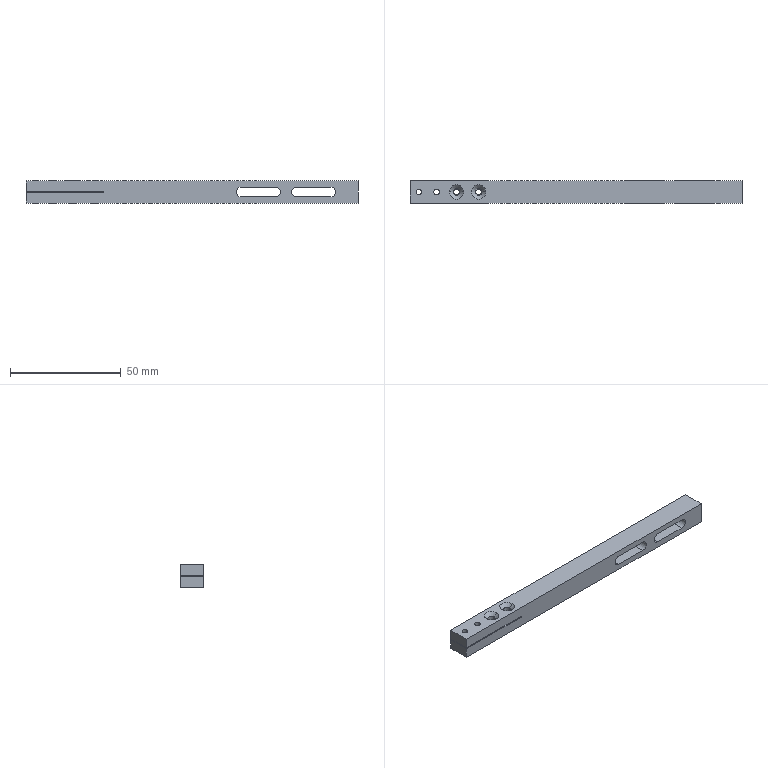Part | NX | features BREP 1 | 1 solid | 38 faces | box 150 x 10 x 10 mm | volume 12850 mm3 | cylinder 20 | plane 14 | cone 4 | commonest cylinder face diameters 2.5 x12 3.4 x4 4.5 x4
STEP:
#1=CARTESIAN_POINT('',(-64.25,0.,0.25));
#2=VERTEX_POINT('',#1);
#3=CARTESIAN_POINT('',(-61.75,0.,0.25));
#4=VERTEX_POINT('',#3);
#5=CARTESIAN_POINT('',(-63.,0.,0.25));
#6=DIRECTION('',(0.,0.,1.));
#7=DIRECTION('',(1.,0.,0.));
#8=AXIS2_PLACEMENT_3D('',#5,#6,#7);
#9=CIRCLE('',#8,1.25);
#10=EDGE_CURVE('',#2,#4,#9,.T.);
#11=ORIENTED_EDGE('',*,*,#10,.F.);
#12=CARTESIAN_POINT('',(-64.25,0.,5.));
#13=VERTEX_POINT('',#12);
#14=CARTESIAN_POINT('',(-64.25,0.,5.));
#15=DIRECTION('',(0.,0.,1.));
#16=VECTOR('',#15,1000.);
#17=LINE('',#14,#16);
#18=EDGE_CURVE('',#2,#13,#17,.T.);
#19=ORIENTED_EDGE('',*,*,#18,.T.);
#20=CARTESIAN_POINT('',(-61.75,0.,5.));
#21=VERTEX_POINT('',#20);
#22=CARTESIAN_POINT('',(-63.,0.,5.));
#23=DIRECTION('',(0.,0.,1.));
#24=DIRECTION('',(1.,0.,0.));
#25=AXIS2_PLACEMENT_3D('',#22,#23,#24);
#26=CIRCLE('',#25,1.25);
#27=EDGE_CURVE('',#13,#21,#26,.T.);
#28=ORIENTED_EDGE('',*,*,#27,.T.);
#29=CARTESIAN_POINT('',(-61.75,0.,5.));
#30=DIRECTION('',(0.,0.,1.));
#31=VECTOR('',#30,1000.);
#32=LINE('',#29,#31);
#33=EDGE_CURVE('',#4,#21,#32,.T.);
#34=ORIENTED_EDGE('',*,*,#33,.F.);
#35=EDGE_LOOP('',(#11,#19,#28,#34));
#36=FACE_BOUND('',#35,.T.);
#37=CARTESIAN_POINT('',(-63.,0.,5.));
#38=DIRECTION('',(0.,0.,1.));
#39=DIRECTION('',(-1.,0.,0.));
#40=AXIS2_PLACEMENT_3D('',#37,#38,#39);
#41=CYLINDRICAL_SURFACE('',#40,1.25);
#42=ADVANCED_FACE('',(#36),#41,.F.);
#43=CARTESIAN_POINT('',(-64.25,0.,-5.));
#44=VERTEX_POINT('',#43);
#45=CARTESIAN_POINT('',(-61.75,0.,-5.));
#46=VERTEX_POINT('',#45);
#47=CARTESIAN_POINT('',(-63.,0.,-5.));
#48=DIRECTION('',(0.,0.,1.));
#49=DIRECTION('',(1.,0.,0.));
#50=AXIS2_PLACEMENT_3D('',#47,#48,#49);
#51=CIRCLE('',#50,1.25);
#52=EDGE_CURVE('',#44,#46,#51,.T.);
#53=ORIENTED_EDGE('',*,*,#52,.F.);
#54=CARTESIAN_POINT('',(-64.25,0.,-0.25));
#55=VERTEX_POINT('',#54);
#56=CARTESIAN_POINT('',(-64.25,0.,5.));
#57=DIRECTION('',(0.,0.,1.));
#58=VECTOR('',#57,1000.);
#59=LINE('',#56,#58);
#60=EDGE_CURVE('',#44,#55,#59,.T.);
#61=ORIENTED_EDGE('',*,*,#60,.T.);
#62=CARTESIAN_POINT('',(-61.75,0.,-0.25));
#63=VERTEX_POINT('',#62);
#64=CARTESIAN_POINT('',(-63.,0.,-0.25));
#65=DIRECTION('',(0.,0.,-1.));
#66=DIRECTION('',(-1.,0.,0.));
#67=AXIS2_PLACEMENT_3D('',#64,#65,#66);
#68=CIRCLE('',#67,1.25);
#69=EDGE_CURVE('',#63,#55,#68,.T.);
#70=ORIENTED_EDGE('',*,*,#69,.F.);
#71=CARTESIAN_POINT('',(-61.75,0.,5.));
#72=DIRECTION('',(0.,0.,1.));
#73=VECTOR('',#72,1000.);
#74=LINE('',#71,#73);
#75=EDGE_CURVE('',#46,#63,#74,.T.);
#76=ORIENTED_EDGE('',*,*,#75,.F.);
#77=EDGE_LOOP('',(#53,#61,#70,#76));
#78=FACE_BOUND('',#77,.T.);
#79=CARTESIAN_POINT('',(-63.,0.,5.));
#80=DIRECTION('',(0.,0.,1.));
#81=DIRECTION('',(-1.,0.,0.));
#82=AXIS2_PLACEMENT_3D('',#79,#80,#81);
#83=CYLINDRICAL_SURFACE('',#82,1.25);
#84=ADVANCED_FACE('',(#78),#83,.F.);
#85=CARTESIAN_POINT('',(-72.25,0.,0.25));
#86=VERTEX_POINT('',#85);
#87=CARTESIAN_POINT('',(-69.75,0.,0.25));
#88=VERTEX_POINT('',#87);
#89=CARTESIAN_POINT('',(-71.,0.,0.25));
#90=DIRECTION('',(0.,0.,1.));
#91=DIRECTION('',(1.,0.,0.));
#92=AXIS2_PLACEMENT_3D('',#89,#90,#91);
#93=CIRCLE('',#92,1.25);
#94=EDGE_CURVE('',#86,#88,#93,.T.);
#95=ORIENTED_EDGE('',*,*,#94,.F.);
#96=CARTESIAN_POINT('',(-72.25,0.,5.));
#97=VERTEX_POINT('',#96);
#98=CARTESIAN_POINT('',(-72.25,0.,5.));
#99=DIRECTION('',(0.,0.,1.));
#100=VECTOR('',#99,1000.);
#101=LINE('',#98,#100);
#102=EDGE_CURVE('',#86,#97,#101,.T.);
#103=ORIENTED_EDGE('',*,*,#102,.T.);
#104=CARTESIAN_POINT('',(-69.75,0.,5.));
#105=VERTEX_POINT('',#104);
#106=CARTESIAN_POINT('',(-71.,0.,5.));
#107=DIRECTION('',(0.,0.,1.));
#108=DIRECTION('',(1.,0.,0.));
#109=AXIS2_PLACEMENT_3D('',#106,#107,#108);
#110=CIRCLE('',#109,1.25);
#111=EDGE_CURVE('',#97,#105,#110,.T.);
#112=ORIENTED_EDGE('',*,*,#111,.T.);
#113=CARTESIAN_POINT('',(-69.75,0.,5.));
#114=DIRECTION('',(0.,0.,1.));
#115=VECTOR('',#114,1000.);
#116=LINE('',#113,#115);
#117=EDGE_CURVE('',#88,#105,#116,.T.);
#118=ORIENTED_EDGE('',*,*,#117,.F.);
#119=EDGE_LOOP('',(#95,#103,#112,#118));
#120=FACE_BOUND('',#119,.T.);
#121=CARTESIAN_POINT('',(-71.,0.,5.));
#122=DIRECTION('',(0.,0.,1.));
#123=DIRECTION('',(-1.,0.,0.));
#124=AXIS2_PLACEMENT_3D('',#121,#122,#123);
#125=CYLINDRICAL_SURFACE('',#124,1.25);
#126=ADVANCED_FACE('',(#120),#125,.F.);
#127=CARTESIAN_POINT('',(-72.25,0.,-5.));
#128=VERTEX_POINT('',#127);
#129=CARTESIAN_POINT('',(-69.75,0.,-5.));
#130=VERTEX_POINT('',#129);
#131=CARTESIAN_POINT('',(-71.,0.,-5.));
#132=DIRECTION('',(0.,0.,1.));
#133=DIRECTION('',(1.,0.,0.));
#134=AXIS2_PLACEMENT_3D('',#131,#132,#133);
#135=CIRCLE('',#134,1.25);
#136=EDGE_CURVE('',#128,#130,#135,.T.);
#137=ORIENTED_EDGE('',*,*,#136,.F.);
#138=CARTESIAN_POINT('',(-72.25,0.,-0.25));
#139=VERTEX_POINT('',#138);
#140=CARTESIAN_POINT('',(-72.25,0.,5.));
#141=DIRECTION('',(0.,0.,1.));
#142=VECTOR('',#141,1000.);
#143=LINE('',#140,#142);
#144=EDGE_CURVE('',#128,#139,#143,.T.);
#145=ORIENTED_EDGE('',*,*,#144,.T.);
#146=CARTESIAN_POINT('',(-69.75,0.,-0.25));
#147=VERTEX_POINT('',#146);
#148=CARTESIAN_POINT('',(-71.,0.,-0.25));
#149=DIRECTION('',(0.,0.,-1.));
#150=DIRECTION('',(-1.,0.,0.));
#151=AXIS2_PLACEMENT_3D('',#148,#149,#150);
#152=CIRCLE('',#151,1.25);
#153=EDGE_CURVE('',#147,#139,#152,.T.);
#154=ORIENTED_EDGE('',*,*,#153,.F.);
#155=CARTESIAN_POINT('',(-69.75,0.,5.));
#156=DIRECTION('',(0.,0.,1.));
#157=VECTOR('',#156,1000.);
#158=LINE('',#155,#157);
#159=EDGE_CURVE('',#130,#147,#158,.T.);
#160=ORIENTED_EDGE('',*,*,#159,.F.);
#161=EDGE_LOOP('',(#137,#145,#154,#160));
#162=FACE_BOUND('',#161,.T.);
#163=CARTESIAN_POINT('',(-71.,0.,5.));
#164=DIRECTION('',(0.,0.,1.));
#165=DIRECTION('',(-1.,0.,0.));
#166=AXIS2_PLACEMENT_3D('',#163,#164,#165);
#167=CYLINDRICAL_SURFACE('',#166,1.25);
#168=ADVANCED_FACE('',(#162),#167,.F.);
#169=CARTESIAN_POINT('',(-55.25,0.,-5.));
#170=VERTEX_POINT('',#169);
#171=CARTESIAN_POINT('',(-52.75,0.,-5.));
#172=VERTEX_POINT('',#171);
#173=CARTESIAN_POINT('',(-54.,0.,-5.));
#174=DIRECTION('',(0.,0.,1.));
#175=DIRECTION('',(1.,0.,0.));
#176=AXIS2_PLACEMENT_3D('',#173,#174,#175);
#177=CIRCLE('',#176,1.25);
#178=EDGE_CURVE('',#170,#172,#177,.T.);
#179=ORIENTED_EDGE('',*,*,#178,.F.);
#180=CARTESIAN_POINT('',(-55.25,0.,-0.25));
#181=VERTEX_POINT('',#180);
#182=CARTESIAN_POINT('',(-55.25,0.,5.));
#183=DIRECTION('',(0.,0.,1.));
#184=VECTOR('',#183,1000.);
#185=LINE('',#182,#184);
#186=EDGE_CURVE('',#170,#181,#185,.T.);
#187=ORIENTED_EDGE('',*,*,#186,.T.);
#188=CARTESIAN_POINT('',(-52.75,0.,-0.25));
#189=VERTEX_POINT('',#188);
#190=CARTESIAN_POINT('',(-54.,0.,-0.25));
#191=DIRECTION('',(0.,0.,-1.));
#192=DIRECTION('',(-1.,0.,0.));
#193=AXIS2_PLACEMENT_3D('',#190,#191,#192);
#194=CIRCLE('',#193,1.25);
#195=EDGE_CURVE('',#189,#181,#194,.T.);
#196=ORIENTED_EDGE('',*,*,#195,.F.);
#197=CARTESIAN_POINT('',(-52.75,0.,5.));
#198=DIRECTION('',(0.,0.,1.));
#199=VECTOR('',#198,1000.);
#200=LINE('',#197,#199);
#201=EDGE_CURVE('',#172,#189,#200,.T.);
#202=ORIENTED_EDGE('',*,*,#201,.F.);
#203=EDGE_LOOP('',(#179,#187,#196,#202));
#204=FACE_BOUND('',#203,.T.);
#205=CARTESIAN_POINT('',(-54.,0.,5.));
#206=DIRECTION('',(0.,0.,1.));
#207=DIRECTION('',(-1.,0.,0.));
#208=AXIS2_PLACEMENT_3D('',#205,#206,#207);
#209=CYLINDRICAL_SURFACE('',#208,1.25);
#210=ADVANCED_FACE('',(#204),#209,.F.);
#211=CARTESIAN_POINT('',(-45.25,0.,-5.));
#212=VERTEX_POINT('',#211);
#213=CARTESIAN_POINT('',(-42.75,0.,-5.));
#214=VERTEX_POINT('',#213);
#215=CARTESIAN_POINT('',(-44.,0.,-5.));
#216=DIRECTION('',(0.,0.,1.));
#217=DIRECTION('',(1.,0.,0.));
#218=AXIS2_PLACEMENT_3D('',#215,#216,#217);
#219=CIRCLE('',#218,1.25);
#220=EDGE_CURVE('',#212,#214,#219,.T.);
#221=ORIENTED_EDGE('',*,*,#220,.F.);
#222=CARTESIAN_POINT('',(-45.25,0.,-0.25));
#223=VERTEX_POINT('',#222);
#224=CARTESIAN_POINT('',(-45.25,0.,5.));
#225=DIRECTION('',(0.,0.,1.));
#226=VECTOR('',#225,1000.);
#227=LINE('',#224,#226);
#228=EDGE_CURVE('',#212,#223,#227,.T.);
#229=ORIENTED_EDGE('',*,*,#228,.T.);
#230=CARTESIAN_POINT('',(-42.75,0.,-0.25));
#231=VERTEX_POINT('',#230);
#232=CARTESIAN_POINT('',(-44.,0.,-0.25));
#233=DIRECTION('',(0.,0.,-1.));
#234=DIRECTION('',(-1.,0.,0.));
#235=AXIS2_PLACEMENT_3D('',#232,#233,#234);
#236=CIRCLE('',#235,1.25);
#237=EDGE_CURVE('',#231,#223,#236,.T.);
#238=ORIENTED_EDGE('',*,*,#237,.F.);
#239=CARTESIAN_POINT('',(-42.75,0.,5.));
#240=DIRECTION('',(0.,0.,1.));
#241=VECTOR('',#240,1000.);
#242=LINE('',#239,#241);
#243=EDGE_CURVE('',#214,#231,#242,.T.);
#244=ORIENTED_EDGE('',*,*,#243,.F.);
#245=EDGE_LOOP('',(#221,#229,#238,#244));
#246=FACE_BOUND('',#245,.T.);
#247=CARTESIAN_POINT('',(-44.,0.,5.));
#248=DIRECTION('',(0.,0.,1.));
#249=DIRECTION('',(-1.,0.,0.));
#250=AXIS2_PLACEMENT_3D('',#247,#248,#249);
#251=CYLINDRICAL_SURFACE('',#250,1.25);
#252=ADVANCED_FACE('',(#246),#251,.F.);
#253=CARTESIAN_POINT('',(-55.7,0.,3.4));
#254=VERTEX_POINT('',#253);
#255=CARTESIAN_POINT('',(-52.3,0.,3.4));
#256=VERTEX_POINT('',#255);
#257=CARTESIAN_POINT('',(-54.,0.,3.4));
#258=DIRECTION('',(0.,0.,1.));
#259=DIRECTION('',(1.,0.,0.));
#260=AXIS2_PLACEMENT_3D('',#257,#258,#259);
#261=CIRCLE('',#260,1.7);
#262=EDGE_CURVE('',#254,#256,#261,.T.);
#263=ORIENTED_EDGE('',*,*,#262,.F.);
#264=CARTESIAN_POINT('',(-57.3,0.,5.));
#265=VERTEX_POINT('',#264);
#266=CARTESIAN_POINT('',(-57.3,0.,5.));
#267=DIRECTION('',(-0.7071,0.,0.7071));
#268=VECTOR('',#267,1000.);
#269=LINE('',#266,#268);
#270=EDGE_CURVE('',#254,#265,#269,.T.);
#271=ORIENTED_EDGE('',*,*,#270,.T.);
#272=CARTESIAN_POINT('',(-50.7,0.,5.));
#273=VERTEX_POINT('',#272);
#274=CARTESIAN_POINT('',(-54.,0.,5.));
#275=DIRECTION('',(0.,0.,1.));
#276=DIRECTION('',(1.,0.,0.));
#277=AXIS2_PLACEMENT_3D('',#274,#275,#276);
#278=CIRCLE('',#277,3.3);
#279=EDGE_CURVE('',#265,#273,#278,.T.);
#280=ORIENTED_EDGE('',*,*,#279,.T.);
#281=CARTESIAN_POINT('',(-50.7,0.,5.));
#282=DIRECTION('',(0.7071,0.,0.7071));
#283=VECTOR('',#282,1000.);
#284=LINE('',#281,#283);
#285=EDGE_CURVE('',#256,#273,#284,.T.);
#286=ORIENTED_EDGE('',*,*,#285,.F.);
#287=EDGE_LOOP('',(#263,#271,#280,#286));
#288=FACE_BOUND('',#287,.T.);
#289=CARTESIAN_POINT('',(-54.,0.,5.));
#290=DIRECTION('',(0.,0.,1.));
#291=DIRECTION('',(-1.,0.,0.));
#292=AXIS2_PLACEMENT_3D('',#289,#290,#291);
#293=CONICAL_SURFACE('',#292,3.3,0.7854);
#294=ADVANCED_FACE('',(#288),#293,.F.);
#295=CARTESIAN_POINT('',(-55.7,0.,0.25));
#296=VERTEX_POINT('',#295);
#297=CARTESIAN_POINT('',(-52.3,0.,0.25));
#298=VERTEX_POINT('',#297);
#299=CARTESIAN_POINT('',(-54.,0.,0.25));
#300=DIRECTION('',(0.,0.,1.));
#301=DIRECTION('',(1.,0.,0.));
#302=AXIS2_PLACEMENT_3D('',#299,#300,#301);
#303=CIRCLE('',#302,1.7);
#304=EDGE_CURVE('',#296,#298,#303,.T.);
#305=ORIENTED_EDGE('',*,*,#304,.F.);
#306=CARTESIAN_POINT('',(-55.7,0.,5.));
#307=DIRECTION('',(0.,0.,1.));
#308=VECTOR('',#307,1000.);
#309=LINE('',#306,#308);
#310=EDGE_CURVE('',#296,#254,#309,.T.);
#311=ORIENTED_EDGE('',*,*,#310,.T.);
#312=ORIENTED_EDGE('',*,*,#262,.T.);
#313=CARTESIAN_POINT('',(-52.3,0.,5.));
#314=DIRECTION('',(0.,0.,1.));
#315=VECTOR('',#314,1000.);
#316=LINE('',#313,#315);
#317=EDGE_CURVE('',#298,#256,#316,.T.);
#318=ORIENTED_EDGE('',*,*,#317,.F.);
#319=EDGE_LOOP('',(#305,#311,#312,#318));
#320=FACE_BOUND('',#319,.T.);
#321=CARTESIAN_POINT('',(-54.,0.,5.));
#322=DIRECTION('',(0.,0.,1.));
#323=DIRECTION('',(-1.,0.,0.));
#324=AXIS2_PLACEMENT_3D('',#321,#322,#323);
#325=CYLINDRICAL_SURFACE('',#324,1.7);
#326=ADVANCED_FACE('',(#320),#325,.F.);
#327=CARTESIAN_POINT('',(-45.7,0.,3.4));
#328=VERTEX_POINT('',#327);
#329=CARTESIAN_POINT('',(-42.3,0.,3.4));
#330=VERTEX_POINT('',#329);
#331=CARTESIAN_POINT('',(-44.,0.,3.4));
#332=DIRECTION('',(0.,0.,1.));
#333=DIRECTION('',(1.,0.,0.));
#334=AXIS2_PLACEMENT_3D('',#331,#332,#333);
#335=CIRCLE('',#334,1.7);
#336=EDGE_CURVE('',#328,#330,#335,.T.);
#337=ORIENTED_EDGE('',*,*,#336,.F.);
#338=CARTESIAN_POINT('',(-47.3,0.,5.));
#339=VERTEX_POINT('',#338);
#340=CARTESIAN_POINT('',(-47.3,0.,5.));
#341=DIRECTION('',(-0.7071,0.,0.7071));
#342=VECTOR('',#341,1000.);
#343=LINE('',#340,#342);
#344=EDGE_CURVE('',#328,#339,#343,.T.);
#345=ORIENTED_EDGE('',*,*,#344,.T.);
#346=CARTESIAN_POINT('',(-40.7,0.,5.));
#347=VERTEX_POINT('',#346);
#348=CARTESIAN_POINT('',(-44.,0.,5.));
#349=DIRECTION('',(0.,0.,1.));
#350=DIRECTION('',(1.,0.,0.));
#351=AXIS2_PLACEMENT_3D('',#348,#349,#350);
#352=CIRCLE('',#351,3.3);
#353=EDGE_CURVE('',#339,#347,#352,.T.);
#354=ORIENTED_EDGE('',*,*,#353,.T.);
#355=CARTESIAN_POINT('',(-40.7,0.,5.));
#356=DIRECTION('',(0.7071,0.,0.7071));
#357=VECTOR('',#356,1000.);
#358=LINE('',#355,#357);
#359=EDGE_CURVE('',#330,#347,#358,.T.);
#360=ORIENTED_EDGE('',*,*,#359,.F.);
#361=EDGE_LOOP('',(#337,#345,#354,#360));
#362=FACE_BOUND('',#361,.T.);
#363=CARTESIAN_POINT('',(-44.,0.,5.));
#364=DIRECTION('',(0.,0.,1.));
#365=DIRECTION('',(-1.,0.,0.));
#366=AXIS2_PLACEMENT_3D('',#363,#364,#365);
#367=CONICAL_SURFACE('',#366,3.3,0.7854);
#368=ADVANCED_FACE('',(#362),#367,.F.);
#369=CARTESIAN_POINT('',(-45.7,0.,0.25));
#370=VERTEX_POINT('',#369);
#371=CARTESIAN_POINT('',(-42.3,0.,0.25));
#372=VERTEX_POINT('',#371);
#373=CARTESIAN_POINT('',(-44.,0.,0.25));
#374=DIRECTION('',(0.,0.,1.));
#375=DIRECTION('',(1.,0.,0.));
#376=AXIS2_PLACEMENT_3D('',#373,#374,#375);
#377=CIRCLE('',#376,1.7);
#378=EDGE_CURVE('',#370,#372,#377,.T.);
#379=ORIENTED_EDGE('',*,*,#378,.F.);
#380=CARTESIAN_POINT('',(-45.7,0.,5.));
#381=DIRECTION('',(0.,0.,1.));
#382=VECTOR('',#381,1000.);
#383=LINE('',#380,#382);
#384=EDGE_CURVE('',#370,#328,#383,.T.);
#385=ORIENTED_EDGE('',*,*,#384,.T.);
#386=ORIENTED_EDGE('',*,*,#336,.T.);
#387=CARTESIAN_POINT('',(-42.3,0.,5.));
#388=DIRECTION('',(0.,0.,1.));
#389=VECTOR('',#388,1000.);
#390=LINE('',#387,#389);
#391=EDGE_CURVE('',#372,#330,#390,.T.);
#392=ORIENTED_EDGE('',*,*,#391,.F.);
#393=EDGE_LOOP('',(#379,#385,#386,#392));
#394=FACE_BOUND('',#393,.T.);
#395=CARTESIAN_POINT('',(-44.,0.,5.));
#396=DIRECTION('',(0.,0.,1.));
#397=DIRECTION('',(-1.,0.,0.));
#398=AXIS2_PLACEMENT_3D('',#395,#396,#397);
#399=CYLINDRICAL_SURFACE('',#398,1.7);
#400=ADVANCED_FACE('',(#394),#399,.F.);
#401=CARTESIAN_POINT('',(47.25,5.,2.25));
#402=VERTEX_POINT('',#401);
#403=CARTESIAN_POINT('',(62.75,5.,2.25));
#404=VERTEX_POINT('',#403);
#405=CARTESIAN_POINT('',(47.25,5.,2.25));
#406=DIRECTION('',(1.,0.,0.));
#407=VECTOR('',#406,1000.);
#408=LINE('',#405,#407);
#409=EDGE_CURVE('',#402,#404,#408,.T.);
#410=ORIENTED_EDGE('',*,*,#409,.F.);
#411=CARTESIAN_POINT('',(47.25,5.,-2.25));
#412=VERTEX_POINT('',#411);
#413=CARTESIAN_POINT('',(47.25,5.,0.));
#414=DIRECTION('',(0.,1.,0.));
#415=DIRECTION('',(0.,0.,1.));
#416=AXIS2_PLACEMENT_3D('',#413,#414,#415);
#417=CIRCLE('',#416,2.25);
#418=EDGE_CURVE('',#412,#402,#417,.T.);
#419=ORIENTED_EDGE('',*,*,#418,.F.);
#420=CARTESIAN_POINT('',(62.75,5.,-2.25));
#421=VERTEX_POINT('',#420);
#422=CARTESIAN_POINT('',(47.25,5.,-2.25));
#423=DIRECTION('',(1.,0.,0.));
#424=VECTOR('',#423,1000.);
#425=LINE('',#422,#424);
#426=EDGE_CURVE('',#412,#421,#425,.T.);
#427=ORIENTED_EDGE('',*,*,#426,.T.);
#428=CARTESIAN_POINT('',(62.75,5.,0.));
#429=DIRECTION('',(0.,1.,0.));
#430=DIRECTION('',(0.,0.,1.));
#431=AXIS2_PLACEMENT_3D('',#428,#429,#430);
#432=CIRCLE('',#431,2.25);
#433=EDGE_CURVE('',#404,#421,#432,.T.);
#434=ORIENTED_EDGE('',*,*,#433,.F.);
#435=EDGE_LOOP('',(#410,#419,#427,#434));
#436=FACE_BOUND('',#435,.T.);
#437=CARTESIAN_POINT('',(-75.,5.,-0.25));
#438=VERTEX_POINT('',#437);
#439=CARTESIAN_POINT('',(-75.,5.,-5.));
#440=VERTEX_POINT('',#439);
#441=CARTESIAN_POINT('',(-75.,5.,5.));
#442=DIRECTION('',(0.,0.,-1.));
#443=VECTOR('',#442,1000.);
#444=LINE('',#441,#443);
#445=EDGE_CURVE('',#438,#440,#444,.T.);
#446=ORIENTED_EDGE('',*,*,#445,.F.);
#447=CARTESIAN_POINT('',(-40.,5.,-0.25));
#448=VERTEX_POINT('',#447);
#449=CARTESIAN_POINT('',(-75.,5.,-0.25));
#450=DIRECTION('',(1.,0.,0.));
#451=VECTOR('',#450,1000.);
#452=LINE('',#449,#451);
#453=EDGE_CURVE('',#438,#448,#452,.T.);
#454=ORIENTED_EDGE('',*,*,#453,.T.);
#455=CARTESIAN_POINT('',(-40.,5.,0.25));
#456=VERTEX_POINT('',#455);
#457=CARTESIAN_POINT('',(-40.,5.,5.));
#458=DIRECTION('',(0.,0.,1.));
#459=VECTOR('',#458,1000.);
#460=LINE('',#457,#459);
#461=EDGE_CURVE('',#448,#456,#460,.T.);
#462=ORIENTED_EDGE('',*,*,#461,.T.);
#463=CARTESIAN_POINT('',(-75.,5.,0.25));
#464=VERTEX_POINT('',#463);
#465=CARTESIAN_POINT('',(-75.,5.,0.25));
#466=DIRECTION('',(-1.,0.,0.));
#467=VECTOR('',#466,1000.);
#468=LINE('',#465,#467);
#469=EDGE_CURVE('',#456,#464,#468,.T.);
#470=ORIENTED_EDGE('',*,*,#469,.T.);
#471=CARTESIAN_POINT('',(-75.,5.,5.));
#472=VERTEX_POINT('',#471);
#473=CARTESIAN_POINT('',(-75.,5.,5.));
#474=DIRECTION('',(0.,0.,-1.));
#475=VECTOR('',#474,1000.);
#476=LINE('',#473,#475);
#477=EDGE_CURVE('',#472,#464,#476,.T.);
#478=ORIENTED_EDGE('',*,*,#477,.F.);
#479=CARTESIAN_POINT('',(75.,5.,5.));
#480=VERTEX_POINT('',#479);
#481=CARTESIAN_POINT('',(-75.,5.,5.));
#482=DIRECTION('',(-1.,0.,0.));
#483=VECTOR('',#482,1000.);
#484=LINE('',#481,#483);
#485=EDGE_CURVE('',#480,#472,#484,.T.);
#486=ORIENTED_EDGE('',*,*,#485,.F.);
#487=CARTESIAN_POINT('',(75.,5.,-5.));
#488=VERTEX_POINT('',#487);
#489=CARTESIAN_POINT('',(75.,5.,5.));
#490=DIRECTION('',(0.,0.,-1.));
#491=VECTOR('',#490,1000.);
#492=LINE('',#489,#491);
#493=EDGE_CURVE('',#480,#488,#492,.T.);
#494=ORIENTED_EDGE('',*,*,#493,.T.);
#495=CARTESIAN_POINT('',(-75.,5.,-5.));
#496=DIRECTION('',(-1.,0.,0.));
#497=VECTOR('',#496,1000.);
#498=LINE('',#495,#497);
#499=EDGE_CURVE('',#488,#440,#498,.T.);
#500=ORIENTED_EDGE('',*,*,#499,.T.);
#501=EDGE_LOOP('',(#446,#454,#462,#470,#478,#486,#494,#500));
#502=FACE_BOUND('',#501,.T.);
#503=CARTESIAN_POINT('',(22.25,5.,2.25));
#504=VERTEX_POINT('',#503);
#505=CARTESIAN_POINT('',(37.75,5.,2.25));
#506=VERTEX_POINT('',#505);
#507=CARTESIAN_POINT('',(22.25,5.,2.25));
#508=DIRECTION('',(1.,0.,0.));
#509=VECTOR('',#508,1000.);
#510=LINE('',#507,#509);
#511=EDGE_CURVE('',#504,#506,#510,.T.);
#512=ORIENTED_EDGE('',*,*,#511,.F.);
#513=CARTESIAN_POINT('',(22.25,5.,-2.25));
#514=VERTEX_POINT('',#513);
#515=CARTESIAN_POINT('',(22.25,5.,0.));
#516=DIRECTION('',(0.,1.,0.));
#517=DIRECTION('',(0.,0.,1.));
#518=AXIS2_PLACEMENT_3D('',#515,#516,#517);
#519=CIRCLE('',#518,2.25);
#520=EDGE_CURVE('',#514,#504,#519,.T.);
#521=ORIENTED_EDGE('',*,*,#520,.F.);
#522=CARTESIAN_POINT('',(37.75,5.,-2.25));
#523=VERTEX_POINT('',#522);
#524=CARTESIAN_POINT('',(22.25,5.,-2.25));
#525=DIRECTION('',(1.,0.,0.));
#526=VECTOR('',#525,1000.);
#527=LINE('',#524,#526);
#528=EDGE_CURVE('',#514,#523,#527,.T.);
#529=ORIENTED_EDGE('',*,*,#528,.T.);
#530=CARTESIAN_POINT('',(37.75,5.,0.));
#531=DIRECTION('',(0.,1.,0.));
#532=DIRECTION('',(0.,0.,1.));
#533=AXIS2_PLACEMENT_3D('',#530,#531,#532);
#534=CIRCLE('',#533,2.25);
#535=EDGE_CURVE('',#506,#523,#534,.T.);
#536=ORIENTED_EDGE('',*,*,#535,.F.);
#537=EDGE_LOOP('',(#512,#521,#529,#536));
#538=FACE_BOUND('',#537,.T.);
#539=CARTESIAN_POINT('',(-75.,5.,5.));
#540=DIRECTION('',(0.,-1.,0.));
#541=DIRECTION('',(0.,0.,1.));
#542=AXIS2_PLACEMENT_3D('',#539,#540,#541);
#543=PLANE('',#542);
#544=ADVANCED_FACE('',(#436,#502,#538),#543,.F.);
#545=CARTESIAN_POINT('',(-75.,-5.,-0.25));
#546=VERTEX_POINT('',#545);
#547=CARTESIAN_POINT('',(-75.,-5.,-5.));
#548=VERTEX_POINT('',#547);
#549=CARTESIAN_POINT('',(-75.,-5.,5.));
#550=DIRECTION('',(0.,0.,-1.));
#551=VECTOR('',#550,1000.);
#552=LINE('',#549,#551);
#553=EDGE_CURVE('',#546,#548,#552,.T.);
#554=ORIENTED_EDGE('',*,*,#553,.F.);
#555=CARTESIAN_POINT('',(-75.,-5.,-0.25));
#556=DIRECTION('',(0.,1.,0.));
#557=VECTOR('',#556,1000.);
#558=LINE('',#555,#557);
#559=EDGE_CURVE('',#546,#438,#558,.T.);
#560=ORIENTED_EDGE('',*,*,#559,.T.);
#561=ORIENTED_EDGE('',*,*,#445,.T.);
#562=CARTESIAN_POINT('',(-75.,5.,-5.));
#563=DIRECTION('',(0.,-1.,0.));
#564=VECTOR('',#563,1000.);
#565=LINE('',#562,#564);
#566=EDGE_CURVE('',#440,#548,#565,.T.);
#567=ORIENTED_EDGE('',*,*,#566,.T.);
#568=EDGE_LOOP('',(#554,#560,#561,#567));
#569=FACE_BOUND('',#568,.T.);
#570=CARTESIAN_POINT('',(-75.,5.,5.));
#571=DIRECTION('',(1.,0.,0.));
#572=DIRECTION('',(0.,-1.,0.));
#573=AXIS2_PLACEMENT_3D('',#570,#571,#572);
#574=PLANE('',#573);
#575=ADVANCED_FACE('',(#569),#574,.F.);
#576=CARTESIAN_POINT('',(75.,-5.,-5.));
#577=VERTEX_POINT('',#576);
#578=CARTESIAN_POINT('',(75.,5.,-5.));
#579=DIRECTION('',(0.,1.,0.));
#580=VECTOR('',#579,1000.);
#581=LINE('',#578,#580);
#582=EDGE_CURVE('',#577,#488,#581,.T.);
#583=ORIENTED_EDGE('',*,*,#582,.T.);
#584=ORIENTED_EDGE('',*,*,#493,.F.);
#585=CARTESIAN_POINT('',(75.,-5.,5.));
#586=VERTEX_POINT('',#585);
#587=CARTESIAN_POINT('',(75.,5.,5.));
#588=DIRECTION('',(0.,1.,0.));
#589=VECTOR('',#588,1000.);
#590=LINE('',#587,#589);
#591=EDGE_CURVE('',#586,#480,#590,.T.);
#592=ORIENTED_EDGE('',*,*,#591,.F.);
#593=CARTESIAN_POINT('',(75.,-5.,5.));
#594=DIRECTION('',(0.,0.,-1.));
#595=VECTOR('',#594,1000.);
#596=LINE('',#593,#595);
#597=EDGE_CURVE('',#586,#577,#596,.T.);
#598=ORIENTED_EDGE('',*,*,#597,.T.);
#599=EDGE_LOOP('',(#583,#584,#592,#598));
#600=FACE_BOUND('',#599,.T.);
#601=CARTESIAN_POINT('',(75.,5.,5.));
#602=DIRECTION('',(-1.,0.,0.));
#603=DIRECTION('',(0.,1.,0.));
#604=AXIS2_PLACEMENT_3D('',#601,#602,#603);
#605=PLANE('',#604);
#606=ADVANCED_FACE('',(#600),#605,.F.);
#607=ORIENTED_EDGE('',*,*,#477,.T.);
#608=CARTESIAN_POINT('',(-75.,-5.,0.25));
#609=VERTEX_POINT('',#608);
#610=CARTESIAN_POINT('',(-75.,-5.,0.25));
#611=DIRECTION('',(0.,1.,0.));
#612=VECTOR('',#611,1000.);
#613=LINE('',#610,#612);
#614=EDGE_CURVE('',#609,#464,#613,.T.);
#615=ORIENTED_EDGE('',*,*,#614,.F.);
#616=CARTESIAN_POINT('',(-75.,-5.,5.));
#617=VERTEX_POINT('',#616);
#618=CARTESIAN_POINT('',(-75.,-5.,5.));
#619=DIRECTION('',(0.,0.,-1.));
#620=VECTOR('',#619,1000.);
#621=LINE('',#618,#620);
#622=EDGE_CURVE('',#617,#609,#621,.T.);
#623=ORIENTED_EDGE('',*,*,#622,.F.);
#624=CARTESIAN_POINT('',(-75.,5.,5.));
#625=DIRECTION('',(0.,-1.,0.));
#626=VECTOR('',#625,1000.);
#627=LINE('',#624,#626);
#628=EDGE_CURVE('',#472,#617,#627,.T.);
#629=ORIENTED_EDGE('',*,*,#628,.F.);
#630=EDGE_LOOP('',(#607,#615,#623,#629));
#631=FACE_BOUND('',#630,.T.);
#632=CARTESIAN_POINT('',(-75.,5.,5.));
#633=DIRECTION('',(1.,0.,0.));
#634=DIRECTION('',(0.,-1.,0.));
#635=AXIS2_PLACEMENT_3D('',#632,#633,#634);
#636=PLANE('',#635);
#637=ADVANCED_FACE('',(#631),#636,.F.);
#638=CARTESIAN_POINT('',(47.25,-5.,-2.25));
#639=VERTEX_POINT('',#638);
#640=CARTESIAN_POINT('',(47.25,-5.,2.25));
#641=VERTEX_POINT('',#640);
#642=CARTESIAN_POINT('',(47.25,-5.,0.));
#643=DIRECTION('',(0.,1.,0.));
#644=DIRECTION('',(0.,0.,1.));
#645=AXIS2_PLACEMENT_3D('',#642,#643,#644);
#646=CIRCLE('',#645,2.25);
#647=EDGE_CURVE('',#639,#641,#646,.T.);
#648=ORIENTED_EDGE('',*,*,#647,.T.);
#649=CARTESIAN_POINT('',(62.75,-5.,2.25));
#650=VERTEX_POINT('',#649);
#651=CARTESIAN_POINT('',(47.25,-5.,2.25));
#652=DIRECTION('',(1.,0.,0.));
#653=VECTOR('',#652,1000.);
#654=LINE('',#651,#653);
#655=EDGE_CURVE('',#641,#650,#654,.T.);
#656=ORIENTED_EDGE('',*,*,#655,.T.);
#657=CARTESIAN_POINT('',(62.75,-5.,-2.25));
#658=VERTEX_POINT('',#657);
#659=CARTESIAN_POINT('',(62.75,-5.,0.));
#660=DIRECTION('',(0.,1.,0.));
#661=DIRECTION('',(0.,0.,1.));
#662=AXIS2_PLACEMENT_3D('',#659,#660,#661);
#663=CIRCLE('',#662,2.25);
#664=EDGE_CURVE('',#650,#658,#663,.T.);
#665=ORIENTED_EDGE('',*,*,#664,.T.);
#666=CARTESIAN_POINT('',(47.25,-5.,-2.25));
#667=DIRECTION('',(1.,0.,0.));
#668=VECTOR('',#667,1000.);
#669=LINE('',#666,#668);
#670=EDGE_CURVE('',#639,#658,#669,.T.);
#671=ORIENTED_EDGE('',*,*,#670,.F.);
#672=EDGE_LOOP('',(#648,#656,#665,#671));
#673=FACE_BOUND('',#672,.T.);
#674=CARTESIAN_POINT('',(22.25,-5.,2.25));
#675=VERTEX_POINT('',#674);
#676=CARTESIAN_POINT('',(37.75,-5.,2.25));
#677=VERTEX_POINT('',#676);
#678=CARTESIAN_POINT('',(22.25,-5.,2.25));
#679=DIRECTION('',(1.,0.,0.));
#680=VECTOR('',#679,1000.);
#681=LINE('',#678,#680);
#682=EDGE_CURVE('',#675,#677,#681,.T.);
#683=ORIENTED_EDGE('',*,*,#682,.T.);
#684=CARTESIAN_POINT('',(37.75,-5.,-2.25));
#685=VERTEX_POINT('',#684);
#686=CARTESIAN_POINT('',(37.75,-5.,0.));
#687=DIRECTION('',(0.,1.,0.));
#688=DIRECTION('',(0.,0.,1.));
#689=AXIS2_PLACEMENT_3D('',#686,#687,#688);
#690=CIRCLE('',#689,2.25);
#691=EDGE_CURVE('',#677,#685,#690,.T.);
#692=ORIENTED_EDGE('',*,*,#691,.T.);
#693=CARTESIAN_POINT('',(22.25,-5.,-2.25));
#694=VERTEX_POINT('',#693);
#695=CARTESIAN_POINT('',(22.25,-5.,-2.25));
#696=DIRECTION('',(1.,0.,0.));
#697=VECTOR('',#696,1000.);
#698=LINE('',#695,#697);
#699=EDGE_CURVE('',#694,#685,#698,.T.);
#700=ORIENTED_EDGE('',*,*,#699,.F.);
#701=CARTESIAN_POINT('',(22.25,-5.,0.));
#702=DIRECTION('',(0.,1.,0.));
#703=DIRECTION('',(0.,0.,1.));
#704=AXIS2_PLACEMENT_3D('',#701,#702,#703);
#705=CIRCLE('',#704,2.25);
#706=EDGE_CURVE('',#694,#675,#705,.T.);
#707=ORIENTED_EDGE('',*,*,#706,.T.);
#708=EDGE_LOOP('',(#683,#692,#700,#707));
#709=FACE_BOUND('',#708,.T.);
#710=CARTESIAN_POINT('',(-40.,-5.,0.25));
#711=VERTEX_POINT('',#710);
#712=CARTESIAN_POINT('',(-40.,-5.,-0.25));
#713=VERTEX_POINT('',#712);
#714=CARTESIAN_POINT('',(-40.,-5.,-0.25));
#715=DIRECTION('',(0.,0.,-1.));
#716=VECTOR('',#715,1000.);
#717=LINE('',#714,#716);
#718=EDGE_CURVE('',#711,#713,#717,.T.);
#719=ORIENTED_EDGE('',*,*,#718,.T.);
#720=CARTESIAN_POINT('',(-75.,-5.,-0.25));
#721=DIRECTION('',(-1.,0.,0.));
#722=VECTOR('',#721,1000.);
#723=LINE('',#720,#722);
#724=EDGE_CURVE('',#713,#546,#723,.T.);
#725=ORIENTED_EDGE('',*,*,#724,.T.);
#726=ORIENTED_EDGE('',*,*,#553,.T.);
#727=CARTESIAN_POINT('',(-75.,-5.,-5.));
#728=DIRECTION('',(1.,0.,0.));
#729=VECTOR('',#728,1000.);
#730=LINE('',#727,#729);
#731=EDGE_CURVE('',#548,#577,#730,.T.);
#732=ORIENTED_EDGE('',*,*,#731,.T.);
#733=ORIENTED_EDGE('',*,*,#597,.F.);
#734=CARTESIAN_POINT('',(-75.,-5.,5.));
#735=DIRECTION('',(1.,0.,0.));
#736=VECTOR('',#735,1000.);
#737=LINE('',#734,#736);
#738=EDGE_CURVE('',#617,#586,#737,.T.);
#739=ORIENTED_EDGE('',*,*,#738,.F.);
#740=ORIENTED_EDGE('',*,*,#622,.T.);
#741=CARTESIAN_POINT('',(-75.,-5.,0.25));
#742=DIRECTION('',(1.,0.,0.));
#743=VECTOR('',#742,1000.);
#744=LINE('',#741,#743);
#745=EDGE_CURVE('',#609,#711,#744,.T.);
#746=ORIENTED_EDGE('',*,*,#745,.T.);
#747=EDGE_LOOP('',(#719,#725,#726,#732,#733,#739,#740,#746));
#748=FACE_BOUND('',#747,.T.);
#749=CARTESIAN_POINT('',(-75.,-5.,5.));
#750=DIRECTION('',(0.,1.,0.));
#751=DIRECTION('',(0.,0.,-1.));
#752=AXIS2_PLACEMENT_3D('',#749,#750,#751);
#753=PLANE('',#752);
#754=ADVANCED_FACE('',(#673,#709,#748),#753,.F.);
#755=CARTESIAN_POINT('',(-63.,0.,5.));
#756=DIRECTION('',(0.,0.,1.));
#757=DIRECTION('',(1.,0.,0.));
#758=AXIS2_PLACEMENT_3D('',#755,#756,#757);
#759=CIRCLE('',#758,1.25);
#760=EDGE_CURVE('',#21,#13,#759,.T.);
#761=ORIENTED_EDGE('',*,*,#760,.F.);
#762=ORIENTED_EDGE('',*,*,#27,.F.);
#763=EDGE_LOOP('',(#761,#762));
#764=FACE_BOUND('',#763,.T.);
#765=CARTESIAN_POINT('',(-71.,0.,5.));
#766=DIRECTION('',(0.,0.,1.));
#767=DIRECTION('',(1.,0.,0.));
#768=AXIS2_PLACEMENT_3D('',#765,#766,#767);
#769=CIRCLE('',#768,1.25);
#770=EDGE_CURVE('',#105,#97,#769,.T.);
#771=ORIENTED_EDGE('',*,*,#770,.F.);
#772=ORIENTED_EDGE('',*,*,#111,.F.);
#773=EDGE_LOOP('',(#771,#772));
#774=FACE_BOUND('',#773,.T.);
#775=CARTESIAN_POINT('',(-54.,0.,5.));
#776=DIRECTION('',(0.,0.,1.));
#777=DIRECTION('',(1.,0.,0.));
#778=AXIS2_PLACEMENT_3D('',#775,#776,#777);
#779=CIRCLE('',#778,3.3);
#780=EDGE_CURVE('',#273,#265,#779,.T.);
#781=ORIENTED_EDGE('',*,*,#780,.F.);
#782=ORIENTED_EDGE('',*,*,#279,.F.);
#783=EDGE_LOOP('',(#781,#782));
#784=FACE_BOUND('',#783,.T.);
#785=CARTESIAN_POINT('',(-44.,0.,5.));
#786=DIRECTION('',(0.,0.,1.));
#787=DIRECTION('',(1.,0.,0.));
#788=AXIS2_PLACEMENT_3D('',#785,#786,#787);
#789=CIRCLE('',#788,3.3);
#790=EDGE_CURVE('',#347,#339,#789,.T.);
#791=ORIENTED_EDGE('',*,*,#790,.F.);
#792=ORIENTED_EDGE('',*,*,#353,.F.);
#793=EDGE_LOOP('',(#791,#792));
#794=FACE_BOUND('',#793,.T.);
#795=ORIENTED_EDGE('',*,*,#591,.T.);
#796=ORIENTED_EDGE('',*,*,#485,.T.);
#797=ORIENTED_EDGE('',*,*,#628,.T.);
#798=ORIENTED_EDGE('',*,*,#738,.T.);
#799=EDGE_LOOP('',(#795,#796,#797,#798));
#800=FACE_BOUND('',#799,.T.);
#801=CARTESIAN_POINT('',(0.,0.,5.));
#802=DIRECTION('',(0.,0.,1.));
#803=DIRECTION('',(-1.,0.,0.));
#804=AXIS2_PLACEMENT_3D('',#801,#802,#803);
#805=PLANE('',#804);
#806=ADVANCED_FACE('',(#764,#774,#784,#794,#800),#805,.T.);
#807=CARTESIAN_POINT('',(-63.,0.,-5.));
#808=DIRECTION('',(0.,0.,1.));
#809=DIRECTION('',(1.,0.,0.));
#810=AXIS2_PLACEMENT_3D('',#807,#808,#809);
#811=CIRCLE('',#810,1.25);
#812=EDGE_CURVE('',#46,#44,#811,.T.);
#813=ORIENTED_EDGE('',*,*,#812,.T.);
#814=ORIENTED_EDGE('',*,*,#52,.T.);
#815=EDGE_LOOP('',(#813,#814));
#816=FACE_BOUND('',#815,.T.);
#817=CARTESIAN_POINT('',(-71.,0.,-5.));
#818=DIRECTION('',(0.,0.,1.));
#819=DIRECTION('',(1.,0.,0.));
#820=AXIS2_PLACEMENT_3D('',#817,#818,#819);
#821=CIRCLE('',#820,1.25);
#822=EDGE_CURVE('',#130,#128,#821,.T.);
#823=ORIENTED_EDGE('',*,*,#822,.T.);
#824=ORIENTED_EDGE('',*,*,#136,.T.);
#825=EDGE_LOOP('',(#823,#824));
#826=FACE_BOUND('',#825,.T.);
#827=CARTESIAN_POINT('',(-54.,0.,-5.));
#828=DIRECTION('',(0.,0.,1.));
#829=DIRECTION('',(1.,0.,0.));
#830=AXIS2_PLACEMENT_3D('',#827,#828,#829);
#831=CIRCLE('',#830,1.25);
#832=EDGE_CURVE('',#172,#170,#831,.T.);
#833=ORIENTED_EDGE('',*,*,#832,.T.);
#834=ORIENTED_EDGE('',*,*,#178,.T.);
#835=EDGE_LOOP('',(#833,#834));
#836=FACE_BOUND('',#835,.T.);
#837=CARTESIAN_POINT('',(-44.,0.,-5.));
#838=DIRECTION('',(0.,0.,1.));
#839=DIRECTION('',(1.,0.,0.));
#840=AXIS2_PLACEMENT_3D('',#837,#838,#839);
#841=CIRCLE('',#840,1.25);
#842=EDGE_CURVE('',#214,#212,#841,.T.);
#843=ORIENTED_EDGE('',*,*,#842,.T.);
#844=ORIENTED_EDGE('',*,*,#220,.T.);
#845=EDGE_LOOP('',(#843,#844));
#846=FACE_BOUND('',#845,.T.);
#847=ORIENTED_EDGE('',*,*,#582,.F.);
#848=ORIENTED_EDGE('',*,*,#731,.F.);
#849=ORIENTED_EDGE('',*,*,#566,.F.);
#850=ORIENTED_EDGE('',*,*,#499,.F.);
#851=EDGE_LOOP('',(#847,#848,#849,#850));
#852=FACE_BOUND('',#851,.T.);
#853=CARTESIAN_POINT('',(0.,0.,-5.));
#854=DIRECTION('',(0.,0.,1.));
#855=DIRECTION('',(-1.,0.,0.));
#856=AXIS2_PLACEMENT_3D('',#853,#854,#855);
#857=PLANE('',#856);
#858=ADVANCED_FACE('',(#816,#826,#836,#846,#852),#857,.F.);
#859=ORIENTED_EDGE('',*,*,#69,.T.);
#860=CARTESIAN_POINT('',(-63.,0.,-0.25));
#861=DIRECTION('',(0.,0.,-1.));
#862=DIRECTION('',(-1.,0.,0.));
#863=AXIS2_PLACEMENT_3D('',#860,#861,#862);
#864=CIRCLE('',#863,1.25);
#865=EDGE_CURVE('',#55,#63,#864,.T.);
#866=ORIENTED_EDGE('',*,*,#865,.T.);
#867=EDGE_LOOP('',(#859,#866));
#868=FACE_BOUND('',#867,.T.);
#869=ORIENTED_EDGE('',*,*,#153,.T.);
#870=CARTESIAN_POINT('',(-71.,0.,-0.25));
#871=DIRECTION('',(0.,0.,-1.));
#872=DIRECTION('',(-1.,0.,0.));
#873=AXIS2_PLACEMENT_3D('',#870,#871,#872);
#874=CIRCLE('',#873,1.25);
#875=EDGE_CURVE('',#139,#147,#874,.T.);
#876=ORIENTED_EDGE('',*,*,#875,.T.);
#877=EDGE_LOOP('',(#869,#876));
#878=FACE_BOUND('',#877,.T.);
#879=ORIENTED_EDGE('',*,*,#195,.T.);
#880=CARTESIAN_POINT('',(-54.,0.,-0.25));
#881=DIRECTION('',(0.,0.,-1.));
#882=DIRECTION('',(-1.,0.,0.));
#883=AXIS2_PLACEMENT_3D('',#880,#881,#882);
#884=CIRCLE('',#883,1.25);
#885=EDGE_CURVE('',#181,#189,#884,.T.);
#886=ORIENTED_EDGE('',*,*,#885,.T.);
#887=EDGE_LOOP('',(#879,#886));
#888=FACE_BOUND('',#887,.T.);
#889=ORIENTED_EDGE('',*,*,#237,.T.);
#890=CARTESIAN_POINT('',(-44.,0.,-0.25));
#891=DIRECTION('',(0.,0.,-1.));
#892=DIRECTION('',(-1.,0.,0.));
#893=AXIS2_PLACEMENT_3D('',#890,#891,#892);
#894=CIRCLE('',#893,1.25);
#895=EDGE_CURVE('',#223,#231,#894,.T.);
#896=ORIENTED_EDGE('',*,*,#895,.T.);
#897=EDGE_LOOP('',(#889,#896));
#898=FACE_BOUND('',#897,.T.);
#899=ORIENTED_EDGE('',*,*,#559,.F.);
#900=ORIENTED_EDGE('',*,*,#724,.F.);
#901=CARTESIAN_POINT('',(-40.,-5.,-0.25));
#902=DIRECTION('',(0.,1.,0.));
#903=VECTOR('',#902,1000.);
#904=LINE('',#901,#903);
#905=EDGE_CURVE('',#713,#448,#904,.T.);
#906=ORIENTED_EDGE('',*,*,#905,.T.);
#907=ORIENTED_EDGE('',*,*,#453,.F.);
#908=EDGE_LOOP('',(#899,#900,#906,#907));
#909=FACE_BOUND('',#908,.T.);
#910=CARTESIAN_POINT('',(-75.,-5.,-0.25));
#911=DIRECTION('',(0.,0.,-1.));
#912=DIRECTION('',(1.,0.,0.));
#913=AXIS2_PLACEMENT_3D('',#910,#911,#912);
#914=PLANE('',#913);
#915=ADVANCED_FACE('',(#868,#878,#888,#898,#909),#914,.F.);
#916=ORIENTED_EDGE('',*,*,#905,.F.);
#917=ORIENTED_EDGE('',*,*,#718,.F.);
#918=CARTESIAN_POINT('',(-40.,-5.,0.25));
#919=DIRECTION('',(0.,1.,0.));
#920=VECTOR('',#919,1000.);
#921=LINE('',#918,#920);
#922=EDGE_CURVE('',#711,#456,#921,.T.);
#923=ORIENTED_EDGE('',*,*,#922,.T.);
#924=ORIENTED_EDGE('',*,*,#461,.F.);
#925=EDGE_LOOP('',(#916,#917,#923,#924));
#926=FACE_BOUND('',#925,.T.);
#927=CARTESIAN_POINT('',(-40.,-5.,-0.25));
#928=DIRECTION('',(1.,0.,0.));
#929=DIRECTION('',(0.,0.,1.));
#930=AXIS2_PLACEMENT_3D('',#927,#928,#929);
#931=PLANE('',#930);
#932=ADVANCED_FACE('',(#926),#931,.F.);
#933=CARTESIAN_POINT('',(-63.,0.,0.25));
#934=DIRECTION('',(0.,0.,1.));
#935=DIRECTION('',(1.,0.,0.));
#936=AXIS2_PLACEMENT_3D('',#933,#934,#935);
#937=CIRCLE('',#936,1.25);
#938=EDGE_CURVE('',#4,#2,#937,.T.);
#939=ORIENTED_EDGE('',*,*,#938,.T.);
#940=ORIENTED_EDGE('',*,*,#10,.T.);
#941=EDGE_LOOP('',(#939,#940));
#942=FACE_BOUND('',#941,.T.);
#943=CARTESIAN_POINT('',(-71.,0.,0.25));
#944=DIRECTION('',(0.,0.,1.));
#945=DIRECTION('',(1.,0.,0.));
#946=AXIS2_PLACEMENT_3D('',#943,#944,#945);
#947=CIRCLE('',#946,1.25);
#948=EDGE_CURVE('',#88,#86,#947,.T.);
#949=ORIENTED_EDGE('',*,*,#948,.T.);
#950=ORIENTED_EDGE('',*,*,#94,.T.);
#951=EDGE_LOOP('',(#949,#950));
#952=FACE_BOUND('',#951,.T.);
#953=CARTESIAN_POINT('',(-54.,0.,0.25));
#954=DIRECTION('',(0.,0.,1.));
#955=DIRECTION('',(1.,0.,0.));
#956=AXIS2_PLACEMENT_3D('',#953,#954,#955);
#957=CIRCLE('',#956,1.7);
#958=EDGE_CURVE('',#298,#296,#957,.T.);
#959=ORIENTED_EDGE('',*,*,#958,.T.);
#960=ORIENTED_EDGE('',*,*,#304,.T.);
#961=EDGE_LOOP('',(#959,#960));
#962=FACE_BOUND('',#961,.T.);
#963=CARTESIAN_POINT('',(-44.,0.,0.25));
#964=DIRECTION('',(0.,0.,1.));
#965=DIRECTION('',(1.,0.,0.));
#966=AXIS2_PLACEMENT_3D('',#963,#964,#965);
#967=CIRCLE('',#966,1.7);
#968=EDGE_CURVE('',#372,#370,#967,.T.);
#969=ORIENTED_EDGE('',*,*,#968,.T.);
#970=ORIENTED_EDGE('',*,*,#378,.T.);
#971=EDGE_LOOP('',(#969,#970));
#972=FACE_BOUND('',#971,.T.);
#973=ORIENTED_EDGE('',*,*,#922,.F.);
#974=ORIENTED_EDGE('',*,*,#745,.F.);
#975=ORIENTED_EDGE('',*,*,#614,.T.);
#976=ORIENTED_EDGE('',*,*,#469,.F.);
#977=EDGE_LOOP('',(#973,#974,#975,#976));
#978=FACE_BOUND('',#977,.T.);
#979=CARTESIAN_POINT('',(-75.,-5.,0.25));
#980=DIRECTION('',(0.,0.,1.));
#981=DIRECTION('',(-1.,0.,0.));
#982=AXIS2_PLACEMENT_3D('',#979,#980,#981);
#983=PLANE('',#982);
#984=ADVANCED_FACE('',(#942,#952,#962,#972,#978),#983,.F.);
#985=ORIENTED_EDGE('',*,*,#384,.F.);
#986=ORIENTED_EDGE('',*,*,#968,.F.);
#987=ORIENTED_EDGE('',*,*,#391,.T.);
#988=CARTESIAN_POINT('',(-44.,0.,3.4));
#989=DIRECTION('',(0.,0.,1.));
#990=DIRECTION('',(1.,0.,0.));
#991=AXIS2_PLACEMENT_3D('',#988,#989,#990);
#992=CIRCLE('',#991,1.7);
#993=EDGE_CURVE('',#330,#328,#992,.T.);
#994=ORIENTED_EDGE('',*,*,#993,.T.);
#995=EDGE_LOOP('',(#985,#986,#987,#994));
#996=FACE_BOUND('',#995,.T.);
#997=CARTESIAN_POINT('',(-44.,0.,5.));
#998=DIRECTION('',(0.,0.,1.));
#999=DIRECTION('',(-1.,0.,0.));
#1000=AXIS2_PLACEMENT_3D('',#997,#998,#999);
#1001=CYLINDRICAL_SURFACE('',#1000,1.7);
#1002=ADVANCED_FACE('',(#996),#1001,.F.);
#1003=ORIENTED_EDGE('',*,*,#344,.F.);
#1004=ORIENTED_EDGE('',*,*,#993,.F.);
#1005=ORIENTED_EDGE('',*,*,#359,.T.);
#1006=ORIENTED_EDGE('',*,*,#790,.T.);
#1007=EDGE_LOOP('',(#1003,#1004,#1005,#1006));
#1008=FACE_BOUND('',#1007,.T.);
#1009=CARTESIAN_POINT('',(-44.,0.,5.));
#1010=DIRECTION('',(0.,0.,1.));
#1011=DIRECTION('',(-1.,0.,0.));
#1012=AXIS2_PLACEMENT_3D('',#1009,#1010,#1011);
#1013=CONICAL_SURFACE('',#1012,3.3,0.7854);
#1014=ADVANCED_FACE('',(#1008),#1013,.F.);
#1015=ORIENTED_EDGE('',*,*,#310,.F.);
#1016=ORIENTED_EDGE('',*,*,#958,.F.);
#1017=ORIENTED_EDGE('',*,*,#317,.T.);
#1018=CARTESIAN_POINT('',(-54.,0.,3.4));
#1019=DIRECTION('',(0.,0.,1.));
#1020=DIRECTION('',(1.,0.,0.));
#1021=AXIS2_PLACEMENT_3D('',#1018,#1019,#1020);
#1022=CIRCLE('',#1021,1.7);
#1023=EDGE_CURVE('',#256,#254,#1022,.T.);
#1024=ORIENTED_EDGE('',*,*,#1023,.T.);
#1025=EDGE_LOOP('',(#1015,#1016,#1017,#1024));
#1026=FACE_BOUND('',#1025,.T.);
#1027=CARTESIAN_POINT('',(-54.,0.,5.));
#1028=DIRECTION('',(0.,0.,1.));
#1029=DIRECTION('',(-1.,0.,0.));
#1030=AXIS2_PLACEMENT_3D('',#1027,#1028,#1029);
#1031=CYLINDRICAL_SURFACE('',#1030,1.7);
#1032=ADVANCED_FACE('',(#1026),#1031,.F.);
#1033=ORIENTED_EDGE('',*,*,#270,.F.);
#1034=ORIENTED_EDGE('',*,*,#1023,.F.);
#1035=ORIENTED_EDGE('',*,*,#285,.T.);
#1036=ORIENTED_EDGE('',*,*,#780,.T.);
#1037=EDGE_LOOP('',(#1033,#1034,#1035,#1036));
#1038=FACE_BOUND('',#1037,.T.);
#1039=CARTESIAN_POINT('',(-54.,0.,5.));
#1040=DIRECTION('',(0.,0.,1.));
#1041=DIRECTION('',(-1.,0.,0.));
#1042=AXIS2_PLACEMENT_3D('',#1039,#1040,#1041);
#1043=CONICAL_SURFACE('',#1042,3.3,0.7854);
#1044=ADVANCED_FACE('',(#1038),#1043,.F.);
#1045=ORIENTED_EDGE('',*,*,#228,.F.);
#1046=ORIENTED_EDGE('',*,*,#842,.F.);
#1047=ORIENTED_EDGE('',*,*,#243,.T.);
#1048=ORIENTED_EDGE('',*,*,#895,.F.);
#1049=EDGE_LOOP('',(#1045,#1046,#1047,#1048));
#1050=FACE_BOUND('',#1049,.T.);
#1051=CARTESIAN_POINT('',(-44.,0.,5.));
#1052=DIRECTION('',(0.,0.,1.));
#1053=DIRECTION('',(-1.,0.,0.));
#1054=AXIS2_PLACEMENT_3D('',#1051,#1052,#1053);
#1055=CYLINDRICAL_SURFACE('',#1054,1.25);
#1056=ADVANCED_FACE('',(#1050),#1055,.F.);
#1057=ORIENTED_EDGE('',*,*,#186,.F.);
#1058=ORIENTED_EDGE('',*,*,#832,.F.);
#1059=ORIENTED_EDGE('',*,*,#201,.T.);
#1060=ORIENTED_EDGE('',*,*,#885,.F.);
#1061=EDGE_LOOP('',(#1057,#1058,#1059,#1060));
#1062=FACE_BOUND('',#1061,.T.);
#1063=CARTESIAN_POINT('',(-54.,0.,5.));
#1064=DIRECTION('',(0.,0.,1.));
#1065=DIRECTION('',(-1.,0.,0.));
#1066=AXIS2_PLACEMENT_3D('',#1063,#1064,#1065);
#1067=CYLINDRICAL_SURFACE('',#1066,1.25);
#1068=ADVANCED_FACE('',(#1062),#1067,.F.);
#1069=ORIENTED_EDGE('',*,*,#144,.F.);
#1070=ORIENTED_EDGE('',*,*,#822,.F.);
#1071=ORIENTED_EDGE('',*,*,#159,.T.);
#1072=ORIENTED_EDGE('',*,*,#875,.F.);
#1073=EDGE_LOOP('',(#1069,#1070,#1071,#1072));
#1074=FACE_BOUND('',#1073,.T.);
#1075=CARTESIAN_POINT('',(-71.,0.,5.));
#1076=DIRECTION('',(0.,0.,1.));
#1077=DIRECTION('',(-1.,0.,0.));
#1078=AXIS2_PLACEMENT_3D('',#1075,#1076,#1077);
#1079=CYLINDRICAL_SURFACE('',#1078,1.25);
#1080=ADVANCED_FACE('',(#1074),#1079,.F.);
#1081=ORIENTED_EDGE('',*,*,#102,.F.);
#1082=ORIENTED_EDGE('',*,*,#948,.F.);
#1083=ORIENTED_EDGE('',*,*,#117,.T.);
#1084=ORIENTED_EDGE('',*,*,#770,.T.);
#1085=EDGE_LOOP('',(#1081,#1082,#1083,#1084));
#1086=FACE_BOUND('',#1085,.T.);
#1087=CARTESIAN_POINT('',(-71.,0.,5.));
#1088=DIRECTION('',(0.,0.,1.));
#1089=DIRECTION('',(-1.,0.,0.));
#1090=AXIS2_PLACEMENT_3D('',#1087,#1088,#1089);
#1091=CYLINDRICAL_SURFACE('',#1090,1.25);
#1092=ADVANCED_FACE('',(#1086),#1091,.F.);
#1093=ORIENTED_EDGE('',*,*,#60,.F.);
#1094=ORIENTED_EDGE('',*,*,#812,.F.);
#1095=ORIENTED_EDGE('',*,*,#75,.T.);
#1096=ORIENTED_EDGE('',*,*,#865,.F.);
#1097=EDGE_LOOP('',(#1093,#1094,#1095,#1096));
#1098=FACE_BOUND('',#1097,.T.);
#1099=CARTESIAN_POINT('',(-63.,0.,5.));
#1100=DIRECTION('',(0.,0.,1.));
#1101=DIRECTION('',(-1.,0.,0.));
#1102=AXIS2_PLACEMENT_3D('',#1099,#1100,#1101);
#1103=CYLINDRICAL_SURFACE('',#1102,1.25);
#1104=ADVANCED_FACE('',(#1098),#1103,.F.);
#1105=ORIENTED_EDGE('',*,*,#18,.F.);
#1106=ORIENTED_EDGE('',*,*,#938,.F.);
#1107=ORIENTED_EDGE('',*,*,#33,.T.);
#1108=ORIENTED_EDGE('',*,*,#760,.T.);
#1109=EDGE_LOOP('',(#1105,#1106,#1107,#1108));
#1110=FACE_BOUND('',#1109,.T.);
#1111=CARTESIAN_POINT('',(-63.,0.,5.));
#1112=DIRECTION('',(0.,0.,1.));
#1113=DIRECTION('',(-1.,0.,0.));
#1114=AXIS2_PLACEMENT_3D('',#1111,#1112,#1113);
#1115=CYLINDRICAL_SURFACE('',#1114,1.25);
#1116=ADVANCED_FACE('',(#1110),#1115,.F.);
#1117=ORIENTED_EDGE('',*,*,#691,.F.);
#1118=CARTESIAN_POINT('',(37.75,5.,2.25));
#1119=DIRECTION('',(0.,-1.,0.));
#1120=VECTOR('',#1119,1000.);
#1121=LINE('',#1118,#1120);
#1122=EDGE_CURVE('',#506,#677,#1121,.T.);
#1123=ORIENTED_EDGE('',*,*,#1122,.F.);
#1124=ORIENTED_EDGE('',*,*,#535,.T.);
#1125=CARTESIAN_POINT('',(37.75,5.,-2.25));
#1126=DIRECTION('',(0.,1.,0.));
#1127=VECTOR('',#1126,1000.);
#1128=LINE('',#1125,#1127);
#1129=EDGE_CURVE('',#685,#523,#1128,.T.);
#1130=ORIENTED_EDGE('',*,*,#1129,.F.);
#1131=EDGE_LOOP('',(#1117,#1123,#1124,#1130));
#1132=FACE_BOUND('',#1131,.T.);
#1133=CARTESIAN_POINT('',(37.75,5.,0.));
#1134=DIRECTION('',(0.,1.,0.));
#1135=DIRECTION('',(0.,0.,-1.));
#1136=AXIS2_PLACEMENT_3D('',#1133,#1134,#1135);
#1137=CYLINDRICAL_SURFACE('',#1136,2.25);
#1138=ADVANCED_FACE('',(#1132),#1137,.F.);
#1139=ORIENTED_EDGE('',*,*,#520,.T.);
#1140=CARTESIAN_POINT('',(22.25,5.,2.25));
#1141=DIRECTION('',(0.,1.,0.));
#1142=VECTOR('',#1141,1000.);
#1143=LINE('',#1140,#1142);
#1144=EDGE_CURVE('',#675,#504,#1143,.T.);
#1145=ORIENTED_EDGE('',*,*,#1144,.F.);
#1146=ORIENTED_EDGE('',*,*,#706,.F.);
#1147=CARTESIAN_POINT('',(22.25,5.,-2.25));
#1148=DIRECTION('',(0.,-1.,0.));
#1149=VECTOR('',#1148,1000.);
#1150=LINE('',#1147,#1149);
#1151=EDGE_CURVE('',#514,#694,#1150,.T.);
#1152=ORIENTED_EDGE('',*,*,#1151,.F.);
#1153=EDGE_LOOP('',(#1139,#1145,#1146,#1152));
#1154=FACE_BOUND('',#1153,.T.);
#1155=CARTESIAN_POINT('',(22.25,5.,0.));
#1156=DIRECTION('',(0.,1.,0.));
#1157=DIRECTION('',(0.,0.,-1.));
#1158=AXIS2_PLACEMENT_3D('',#1155,#1156,#1157);
#1159=CYLINDRICAL_SURFACE('',#1158,2.25);
#1160=ADVANCED_FACE('',(#1154),#1159,.F.);
#1161=ORIENTED_EDGE('',*,*,#1129,.T.);
#1162=ORIENTED_EDGE('',*,*,#528,.F.);
#1163=ORIENTED_EDGE('',*,*,#1151,.T.);
#1164=ORIENTED_EDGE('',*,*,#699,.T.);
#1165=EDGE_LOOP('',(#1161,#1162,#1163,#1164));
#1166=FACE_BOUND('',#1165,.T.);
#1167=CARTESIAN_POINT('',(22.25,5.,-2.25));
#1168=DIRECTION('',(0.,0.,-1.));
#1169=DIRECTION('',(1.,0.,0.));
#1170=AXIS2_PLACEMENT_3D('',#1167,#1168,#1169);
#1171=PLANE('',#1170);
#1172=ADVANCED_FACE('',(#1166),#1171,.F.);
#1173=ORIENTED_EDGE('',*,*,#1122,.T.);
#1174=ORIENTED_EDGE('',*,*,#682,.F.);
#1175=ORIENTED_EDGE('',*,*,#1144,.T.);
#1176=ORIENTED_EDGE('',*,*,#511,.T.);
#1177=EDGE_LOOP('',(#1173,#1174,#1175,#1176));
#1178=FACE_BOUND('',#1177,.T.);
#1179=CARTESIAN_POINT('',(22.25,5.,2.25));
#1180=DIRECTION('',(0.,0.,1.));
#1181=DIRECTION('',(-1.,0.,0.));
#1182=AXIS2_PLACEMENT_3D('',#1179,#1180,#1181);
#1183=PLANE('',#1182);
#1184=ADVANCED_FACE('',(#1178),#1183,.F.);
#1185=ORIENTED_EDGE('',*,*,#664,.F.);
#1186=CARTESIAN_POINT('',(62.75,5.,2.25));
#1187=DIRECTION('',(0.,-1.,0.));
#1188=VECTOR('',#1187,1000.);
#1189=LINE('',#1186,#1188);
#1190=EDGE_CURVE('',#404,#650,#1189,.T.);
#1191=ORIENTED_EDGE('',*,*,#1190,.F.);
#1192=ORIENTED_EDGE('',*,*,#433,.T.);
#1193=CARTESIAN_POINT('',(62.75,5.,-2.25));
#1194=DIRECTION('',(0.,1.,0.));
#1195=VECTOR('',#1194,1000.);
#1196=LINE('',#1193,#1195);
#1197=EDGE_CURVE('',#658,#421,#1196,.T.);
#1198=ORIENTED_EDGE('',*,*,#1197,.F.);
#1199=EDGE_LOOP('',(#1185,#1191,#1192,#1198));
#1200=FACE_BOUND('',#1199,.T.);
#1201=CARTESIAN_POINT('',(62.75,5.,0.));
#1202=DIRECTION('',(0.,1.,0.));
#1203=DIRECTION('',(0.,0.,-1.));
#1204=AXIS2_PLACEMENT_3D('',#1201,#1202,#1203);
#1205=CYLINDRICAL_SURFACE('',#1204,2.25);
#1206=ADVANCED_FACE('',(#1200),#1205,.F.);
#1207=ORIENTED_EDGE('',*,*,#418,.T.);
#1208=CARTESIAN_POINT('',(47.25,5.,2.25));
#1209=DIRECTION('',(0.,1.,0.));
#1210=VECTOR('',#1209,1000.);
#1211=LINE('',#1208,#1210);
#1212=EDGE_CURVE('',#641,#402,#1211,.T.);
#1213=ORIENTED_EDGE('',*,*,#1212,.F.);
#1214=ORIENTED_EDGE('',*,*,#647,.F.);
#1215=CARTESIAN_POINT('',(47.25,5.,-2.25));
#1216=DIRECTION('',(0.,-1.,0.));
#1217=VECTOR('',#1216,1000.);
#1218=LINE('',#1215,#1217);
#1219=EDGE_CURVE('',#412,#639,#1218,.T.);
#1220=ORIENTED_EDGE('',*,*,#1219,.F.);
#1221=EDGE_LOOP('',(#1207,#1213,#1214,#1220));
#1222=FACE_BOUND('',#1221,.T.);
#1223=CARTESIAN_POINT('',(47.25,5.,0.));
#1224=DIRECTION('',(0.,1.,0.));
#1225=DIRECTION('',(0.,0.,-1.));
#1226=AXIS2_PLACEMENT_3D('',#1223,#1224,#1225);
#1227=CYLINDRICAL_SURFACE('',#1226,2.25);
#1228=ADVANCED_FACE('',(#1222),#1227,.F.);
#1229=ORIENTED_EDGE('',*,*,#1197,.T.);
#1230=ORIENTED_EDGE('',*,*,#426,.F.);
#1231=ORIENTED_EDGE('',*,*,#1219,.T.);
#1232=ORIENTED_EDGE('',*,*,#670,.T.);
#1233=EDGE_LOOP('',(#1229,#1230,#1231,#1232));
#1234=FACE_BOUND('',#1233,.T.);
#1235=CARTESIAN_POINT('',(47.25,5.,-2.25));
#1236=DIRECTION('',(0.,0.,-1.));
#1237=DIRECTION('',(1.,0.,0.));
#1238=AXIS2_PLACEMENT_3D('',#1235,#1236,#1237);
#1239=PLANE('',#1238);
#1240=ADVANCED_FACE('',(#1234),#1239,.F.);
#1241=ORIENTED_EDGE('',*,*,#1190,.T.);
#1242=ORIENTED_EDGE('',*,*,#655,.F.);
#1243=ORIENTED_EDGE('',*,*,#1212,.T.);
#1244=ORIENTED_EDGE('',*,*,#409,.T.);
#1245=EDGE_LOOP('',(#1241,#1242,#1243,#1244));
#1246=FACE_BOUND('',#1245,.T.);
#1247=CARTESIAN_POINT('',(47.25,5.,2.25));
#1248=DIRECTION('',(0.,0.,1.));
#1249=DIRECTION('',(-1.,0.,0.));
#1250=AXIS2_PLACEMENT_3D('',#1247,#1248,#1249);
#1251=PLANE('',#1250);
#1252=ADVANCED_FACE('',(#1246),#1251,.F.);
#1253=CLOSED_SHELL('',(#42,#84,#126,#168,#210,#252,#294,#326,#368,#400,#544,#575,#606,#637,#754,#806,#858,#915,#932,#984,#1002,#1014,#1032,#1044,#1056,#1068,#1080,#1092,#1104,#1116,#1138,#1160,#1172,#1184,#1206,#1228,#1240,#1252));
#1254=MANIFOLD_SOLID_BREP('',#1253);
#1255=(LENGTH_UNIT()NAMED_UNIT(*)SI_UNIT(.MILLI.,.METRE.));
#1256=UNCERTAINTY_MEASURE_WITH_UNIT(LENGTH_MEASURE(0.00001),#1255,'','');
#1257=(NAMED_UNIT(*)PLANE_ANGLE_UNIT()SI_UNIT($,.RADIAN.));
#1258=(NAMED_UNIT(*)SI_UNIT($,.STERADIAN.)SOLID_ANGLE_UNIT());
#1259=(GEOMETRIC_REPRESENTATION_CONTEXT(3)GLOBAL_UNCERTAINTY_ASSIGNED_CONTEXT((#1256))GLOBAL_UNIT_ASSIGNED_CONTEXT((#1255,#1257,#1258))REPRESENTATION_CONTEXT('',''));
#1260=ADVANCED_BREP_SHAPE_REPRESENTATION('',(#1254),#1259);